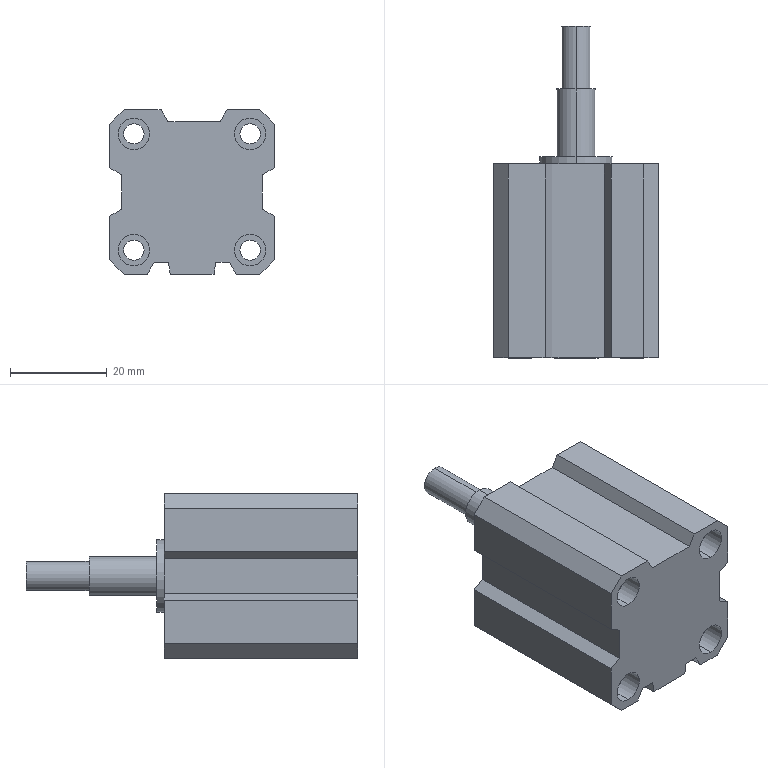Part | NX | 1 solid | 79 faces | box 34 x 68.5 x 34 mm | volume 39955 mm3 | plane 41 | cylinder 34 | cone 4 | commonest cylinder face diameters 6.5 x16 4.2 x8 4.5 x4 6 x2 8 x2 15 x2